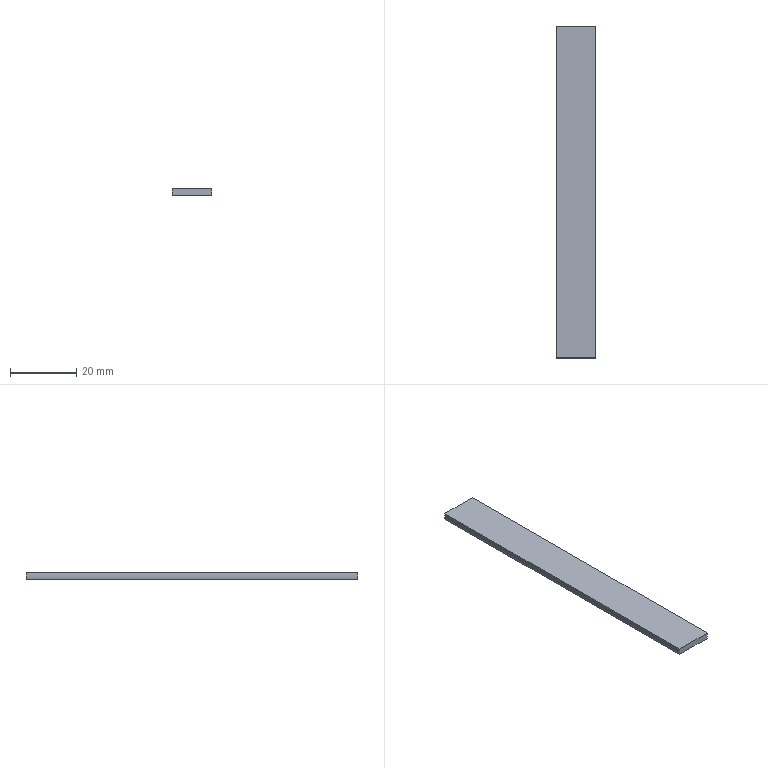Part | STEP file | Cooling fin - upper - Tower - 1 cav | 1 solid | 6 faces | box 12 x 100 x 2 mm | volume 2389 mm3 | plane 4 | cylinder 2 | commonest cylinder face diameters 12 x2
STEP:
#1=CARTESIAN_POINT('',(0.,0.,0.));
#2=DIRECTION('',(0.,0.,1.));
#3=DIRECTION('',(1.,0.,0.));
#4=AXIS2_PLACEMENT_3D('',#1,#2,#3);
#5=CARTESIAN_POINT('',(5.916,0.,-1.));
#6=VERTEX_POINT('',#5);
#7=CARTESIAN_POINT('',(5.916,100.,-1.));
#8=VERTEX_POINT('',#7);
#9=CARTESIAN_POINT('',(5.916,0.,-1.));
#10=DIRECTION('',(0.,1.,0.));
#11=VECTOR('',#10,1.);
#12=LINE('',#9,#11);
#13=CARTESIAN_POINT('',(-10.,100.,-1.));
#14=DIRECTION('',(0.,0.,1.));
#15=DIRECTION('',(1.,0.,0.));
#16=AXIS2_PLACEMENT_3D('',#13,#14,#15);
#17=PLANE('',#16);
#18=CARTESIAN_POINT('',(15.916,-100.));
#19=DIRECTION('',(0.,1.));
#20=VECTOR('',#19,1.);
#21=LINE('',#18,#20);
#22=(GEOMETRIC_REPRESENTATION_CONTEXT(2)PARAMETRIC_REPRESENTATION_CONTEXT()REPRESENTATION_CONTEXT('',''));
#23=DEFINITIONAL_REPRESENTATION('',(#21),#22);
#24=PCURVE('',#17,#23);
#25=CARTESIAN_POINT('',(0.,0.,0.));
#26=DIRECTION('',(0.,1.,0.));
#27=DIRECTION('',(0.,0.,1.));
#28=AXIS2_PLACEMENT_3D('',#25,#26,#27);
#29=CYLINDRICAL_SURFACE('',#28,6.);
#30=CARTESIAN_POINT('',(1.738,0.));
#31=DIRECTION('',(0.,1.));
#32=VECTOR('',#31,1.);
#33=LINE('',#30,#32);
#34=(GEOMETRIC_REPRESENTATION_CONTEXT(2)PARAMETRIC_REPRESENTATION_CONTEXT()REPRESENTATION_CONTEXT('',''));
#35=DEFINITIONAL_REPRESENTATION('',(#33),#34);
#36=PCURVE('',#29,#35);
#37=SURFACE_CURVE('',#12,(#24,#36),.PCURVE_S1.);
#38=EDGE_CURVE('',#6,#8,#37,.T.);
#39=ORIENTED_EDGE('',*,*,#38,.F.);
#40=CARTESIAN_POINT('',(-5.916,0.,-1.));
#41=VERTEX_POINT('',#40);
#42=CARTESIAN_POINT('',(-10.,0.,-1.));
#43=DIRECTION('',(-1.,0.,0.));
#44=VECTOR('',#43,1.);
#45=LINE('',#42,#44);
#46=CARTESIAN_POINT('',(0.,-100.));
#47=DIRECTION('',(-1.,0.));
#48=VECTOR('',#47,1.);
#49=LINE('',#46,#48);
#50=(GEOMETRIC_REPRESENTATION_CONTEXT(2)PARAMETRIC_REPRESENTATION_CONTEXT()REPRESENTATION_CONTEXT('',''));
#51=DEFINITIONAL_REPRESENTATION('',(#49),#50);
#52=PCURVE('',#17,#51);
#53=CARTESIAN_POINT('',(0.,0.,0.));
#54=DIRECTION('',(0.,-1.,0.));
#55=DIRECTION('',(0.,0.,-1.));
#56=AXIS2_PLACEMENT_3D('',#53,#54,#55);
#57=PLANE('',#56);
#58=CARTESIAN_POINT('',(1.,-10.));
#59=DIRECTION('',(0.,-1.));
#60=VECTOR('',#59,1.);
#61=LINE('',#58,#60);
#62=(GEOMETRIC_REPRESENTATION_CONTEXT(2)PARAMETRIC_REPRESENTATION_CONTEXT()REPRESENTATION_CONTEXT('',''));
#63=DEFINITIONAL_REPRESENTATION('',(#61),#62);
#64=PCURVE('',#57,#63);
#65=SURFACE_CURVE('',#45,(#52,#64),.PCURVE_S1.);
#66=EDGE_CURVE('',#6,#41,#65,.T.);
#67=ORIENTED_EDGE('',*,*,#66,.T.);
#68=CARTESIAN_POINT('',(-5.916,100.,-1.));
#69=VERTEX_POINT('',#68);
#70=CARTESIAN_POINT('',(-5.916,0.,-1.));
#71=DIRECTION('',(0.,-1.,0.));
#72=VECTOR('',#71,1.);
#73=LINE('',#70,#72);
#74=CARTESIAN_POINT('',(4.084,-100.));
#75=DIRECTION('',(0.,-1.));
#76=VECTOR('',#75,1.);
#77=LINE('',#74,#76);
#78=(GEOMETRIC_REPRESENTATION_CONTEXT(2)PARAMETRIC_REPRESENTATION_CONTEXT()REPRESENTATION_CONTEXT('',''));
#79=DEFINITIONAL_REPRESENTATION('',(#77),#78);
#80=PCURVE('',#17,#79);
#81=CARTESIAN_POINT('',(0.,0.,0.));
#82=DIRECTION('',(0.,1.,0.));
#83=DIRECTION('',(0.,0.,1.));
#84=AXIS2_PLACEMENT_3D('',#81,#82,#83);
#85=CYLINDRICAL_SURFACE('',#84,6.);
#86=CARTESIAN_POINT('',(4.545,0.));
#87=DIRECTION('',(0.,-1.));
#88=VECTOR('',#87,1.);
#89=LINE('',#86,#88);
#90=(GEOMETRIC_REPRESENTATION_CONTEXT(2)PARAMETRIC_REPRESENTATION_CONTEXT()REPRESENTATION_CONTEXT('',''));
#91=DEFINITIONAL_REPRESENTATION('',(#89),#90);
#92=PCURVE('',#85,#91);
#93=SURFACE_CURVE('',#73,(#80,#92),.PCURVE_S1.);
#94=EDGE_CURVE('',#69,#41,#93,.T.);
#95=ORIENTED_EDGE('',*,*,#94,.F.);
#96=CARTESIAN_POINT('',(-10.,100.,-1.));
#97=DIRECTION('',(-1.,0.,0.));
#98=VECTOR('',#97,1.);
#99=LINE('',#96,#98);
#100=CARTESIAN_POINT('',(0.,0.));
#101=DIRECTION('',(-1.,0.));
#102=VECTOR('',#101,1.);
#103=LINE('',#100,#102);
#104=(GEOMETRIC_REPRESENTATION_CONTEXT(2)PARAMETRIC_REPRESENTATION_CONTEXT()REPRESENTATION_CONTEXT('',''));
#105=DEFINITIONAL_REPRESENTATION('',(#103),#104);
#106=PCURVE('',#17,#105);
#107=CARTESIAN_POINT('',(0.,100.,0.));
#108=DIRECTION('',(0.,-1.,0.));
#109=DIRECTION('',(0.,0.,-1.));
#110=AXIS2_PLACEMENT_3D('',#107,#108,#109);
#111=PLANE('',#110);
#112=CARTESIAN_POINT('',(1.,-10.));
#113=DIRECTION('',(0.,-1.));
#114=VECTOR('',#113,1.);
#115=LINE('',#112,#114);
#116=(GEOMETRIC_REPRESENTATION_CONTEXT(2)PARAMETRIC_REPRESENTATION_CONTEXT()REPRESENTATION_CONTEXT('',''));
#117=DEFINITIONAL_REPRESENTATION('',(#115),#116);
#118=PCURVE('',#111,#117);
#119=SURFACE_CURVE('',#99,(#106,#118),.PCURVE_S1.);
#120=EDGE_CURVE('',#8,#69,#119,.T.);
#121=ORIENTED_EDGE('',*,*,#120,.F.);
#122=EDGE_LOOP('',(#39,#67,#95,#121));
#123=FACE_BOUND('',#122,.T.);
#124=ADVANCED_FACE('',(#123),#17,.F.);
#125=CARTESIAN_POINT('',(-5.916,0.,1.));
#126=VERTEX_POINT('',#125);
#127=CARTESIAN_POINT('',(-5.916,100.,1.));
#128=VERTEX_POINT('',#127);
#129=CARTESIAN_POINT('',(-5.916,0.,1.));
#130=DIRECTION('',(0.,1.,0.));
#131=VECTOR('',#130,1.);
#132=LINE('',#129,#131);
#133=CARTESIAN_POINT('',(-10.,100.,1.));
#134=DIRECTION('',(0.,0.,-1.));
#135=DIRECTION('',(-1.,0.,0.));
#136=AXIS2_PLACEMENT_3D('',#133,#134,#135);
#137=PLANE('',#136);
#138=CARTESIAN_POINT('',(-4.084,-100.));
#139=DIRECTION('',(0.,1.));
#140=VECTOR('',#139,1.);
#141=LINE('',#138,#140);
#142=(GEOMETRIC_REPRESENTATION_CONTEXT(2)PARAMETRIC_REPRESENTATION_CONTEXT()REPRESENTATION_CONTEXT('',''));
#143=DEFINITIONAL_REPRESENTATION('',(#141),#142);
#144=PCURVE('',#137,#143);
#145=CARTESIAN_POINT('',(4.88,0.));
#146=DIRECTION('',(0.,1.));
#147=VECTOR('',#146,1.);
#148=LINE('',#145,#147);
#149=(GEOMETRIC_REPRESENTATION_CONTEXT(2)PARAMETRIC_REPRESENTATION_CONTEXT()REPRESENTATION_CONTEXT('',''));
#150=DEFINITIONAL_REPRESENTATION('',(#148),#149);
#151=PCURVE('',#85,#150);
#152=SURFACE_CURVE('',#132,(#144,#151),.PCURVE_S1.);
#153=EDGE_CURVE('',#126,#128,#152,.T.);
#154=ORIENTED_EDGE('',*,*,#153,.F.);
#155=CARTESIAN_POINT('',(5.916,0.,1.));
#156=VERTEX_POINT('',#155);
#157=CARTESIAN_POINT('',(-10.,0.,1.));
#158=DIRECTION('',(1.,0.,0.));
#159=VECTOR('',#158,1.);
#160=LINE('',#157,#159);
#161=CARTESIAN_POINT('',(0.,-100.));
#162=DIRECTION('',(-1.,0.));
#163=VECTOR('',#162,1.);
#164=LINE('',#161,#163);
#165=(GEOMETRIC_REPRESENTATION_CONTEXT(2)PARAMETRIC_REPRESENTATION_CONTEXT()REPRESENTATION_CONTEXT('',''));
#166=DEFINITIONAL_REPRESENTATION('',(#164),#165);
#167=PCURVE('',#137,#166);
#168=CARTESIAN_POINT('',(-1.,-10.));
#169=DIRECTION('',(0.,1.));
#170=VECTOR('',#169,1.);
#171=LINE('',#168,#170);
#172=(GEOMETRIC_REPRESENTATION_CONTEXT(2)PARAMETRIC_REPRESENTATION_CONTEXT()REPRESENTATION_CONTEXT('',''));
#173=DEFINITIONAL_REPRESENTATION('',(#171),#172);
#174=PCURVE('',#57,#173);
#175=SURFACE_CURVE('',#160,(#167,#174),.PCURVE_S1.);
#176=EDGE_CURVE('',#126,#156,#175,.T.);
#177=ORIENTED_EDGE('',*,*,#176,.T.);
#178=CARTESIAN_POINT('',(5.916,100.,1.));
#179=VERTEX_POINT('',#178);
#180=CARTESIAN_POINT('',(5.916,0.,1.));
#181=DIRECTION('',(0.,-1.,0.));
#182=VECTOR('',#181,1.);
#183=LINE('',#180,#182);
#184=CARTESIAN_POINT('',(-15.916,-100.));
#185=DIRECTION('',(0.,-1.));
#186=VECTOR('',#185,1.);
#187=LINE('',#184,#186);
#188=(GEOMETRIC_REPRESENTATION_CONTEXT(2)PARAMETRIC_REPRESENTATION_CONTEXT()REPRESENTATION_CONTEXT('',''));
#189=DEFINITIONAL_REPRESENTATION('',(#187),#188);
#190=PCURVE('',#137,#189);
#191=CARTESIAN_POINT('',(1.403,0.));
#192=DIRECTION('',(0.,-1.));
#193=VECTOR('',#192,1.);
#194=LINE('',#191,#193);
#195=(GEOMETRIC_REPRESENTATION_CONTEXT(2)PARAMETRIC_REPRESENTATION_CONTEXT()REPRESENTATION_CONTEXT('',''));
#196=DEFINITIONAL_REPRESENTATION('',(#194),#195);
#197=PCURVE('',#29,#196);
#198=SURFACE_CURVE('',#183,(#190,#197),.PCURVE_S1.);
#199=EDGE_CURVE('',#179,#156,#198,.T.);
#200=ORIENTED_EDGE('',*,*,#199,.F.);
#201=CARTESIAN_POINT('',(-10.,100.,1.));
#202=DIRECTION('',(1.,0.,0.));
#203=VECTOR('',#202,1.);
#204=LINE('',#201,#203);
#205=CARTESIAN_POINT('',(0.,0.));
#206=DIRECTION('',(-1.,0.));
#207=VECTOR('',#206,1.);
#208=LINE('',#205,#207);
#209=(GEOMETRIC_REPRESENTATION_CONTEXT(2)PARAMETRIC_REPRESENTATION_CONTEXT()REPRESENTATION_CONTEXT('',''));
#210=DEFINITIONAL_REPRESENTATION('',(#208),#209);
#211=PCURVE('',#137,#210);
#212=CARTESIAN_POINT('',(-1.,-10.));
#213=DIRECTION('',(0.,1.));
#214=VECTOR('',#213,1.);
#215=LINE('',#212,#214);
#216=(GEOMETRIC_REPRESENTATION_CONTEXT(2)PARAMETRIC_REPRESENTATION_CONTEXT()REPRESENTATION_CONTEXT('',''));
#217=DEFINITIONAL_REPRESENTATION('',(#215),#216);
#218=PCURVE('',#111,#217);
#219=SURFACE_CURVE('',#204,(#211,#218),.PCURVE_S1.);
#220=EDGE_CURVE('',#128,#179,#219,.T.);
#221=ORIENTED_EDGE('',*,*,#220,.F.);
#222=EDGE_LOOP('',(#154,#177,#200,#221));
#223=FACE_BOUND('',#222,.T.);
#224=ADVANCED_FACE('',(#223),#137,.F.);
#225=CARTESIAN_POINT('',(0.,100.,0.));
#226=DIRECTION('',(0.,1.,0.));
#227=DIRECTION('',(0.,0.,1.));
#228=AXIS2_PLACEMENT_3D('',#225,#226,#227);
#229=CIRCLE('',#228,6.);
#230=CARTESIAN_POINT('',(-6.,0.));
#231=CARTESIAN_POINT('',(-6.,10.392));
#232=CARTESIAN_POINT('',(3.,5.196));
#233=CARTESIAN_POINT('',(12.,0.));
#234=CARTESIAN_POINT('',(3.,-5.196));
#235=CARTESIAN_POINT('',(-6.,-10.392));
#236=CARTESIAN_POINT('',(-6.,0.));
#237=(BOUNDED_CURVE()B_SPLINE_CURVE(2,(#230,#231,#232,#233,#234,#235,#236),.UNSPECIFIED.,.T.,.F.)B_SPLINE_CURVE_WITH_KNOTS((1,2,2,2,2,1),(-2.094,0.,2.094,4.189,6.283,8.378),.UNSPECIFIED.)CURVE()GEOMETRIC_REPRESENTATION_ITEM()RATIONAL_B_SPLINE_CURVE((1.,0.5,1.,0.5,1.,0.5,1.))REPRESENTATION_ITEM(''));
#238=(GEOMETRIC_REPRESENTATION_CONTEXT(2)PARAMETRIC_REPRESENTATION_CONTEXT()REPRESENTATION_CONTEXT('',''));
#239=DEFINITIONAL_REPRESENTATION('',(#237),#238);
#240=PCURVE('',#111,#239);
#241=CARTESIAN_POINT('',(0.,100.));
#242=DIRECTION('',(1.,0.));
#243=VECTOR('',#242,1.);
#244=LINE('',#241,#243);
#245=(GEOMETRIC_REPRESENTATION_CONTEXT(2)PARAMETRIC_REPRESENTATION_CONTEXT()REPRESENTATION_CONTEXT('',''));
#246=DEFINITIONAL_REPRESENTATION('',(#244),#245);
#247=PCURVE('',#29,#246);
#248=SURFACE_CURVE('',#229,(#240,#247),.PCURVE_S1.);
#249=EDGE_CURVE('',#179,#8,#248,.T.);
#250=ORIENTED_EDGE('',*,*,#249,.T.);
#251=ORIENTED_EDGE('',*,*,#120,.T.);
#252=CARTESIAN_POINT('',(0.,100.,0.));
#253=DIRECTION('',(0.,1.,0.));
#254=DIRECTION('',(0.,0.,1.));
#255=AXIS2_PLACEMENT_3D('',#252,#253,#254);
#256=CIRCLE('',#255,6.);
#257=CARTESIAN_POINT('',(-6.,0.));
#258=CARTESIAN_POINT('',(-6.,10.392));
#259=CARTESIAN_POINT('',(3.,5.196));
#260=CARTESIAN_POINT('',(12.,0.));
#261=CARTESIAN_POINT('',(3.,-5.196));
#262=CARTESIAN_POINT('',(-6.,-10.392));
#263=CARTESIAN_POINT('',(-6.,0.));
#264=(BOUNDED_CURVE()B_SPLINE_CURVE(2,(#257,#258,#259,#260,#261,#262,#263),.UNSPECIFIED.,.T.,.F.)B_SPLINE_CURVE_WITH_KNOTS((1,2,2,2,2,1),(-2.094,0.,2.094,4.189,6.283,8.378),.UNSPECIFIED.)CURVE()GEOMETRIC_REPRESENTATION_ITEM()RATIONAL_B_SPLINE_CURVE((1.,0.5,1.,0.5,1.,0.5,1.))REPRESENTATION_ITEM(''));
#265=(GEOMETRIC_REPRESENTATION_CONTEXT(2)PARAMETRIC_REPRESENTATION_CONTEXT()REPRESENTATION_CONTEXT('',''));
#266=DEFINITIONAL_REPRESENTATION('',(#264),#265);
#267=PCURVE('',#111,#266);
#268=CARTESIAN_POINT('',(0.,100.));
#269=DIRECTION('',(1.,0.));
#270=VECTOR('',#269,1.);
#271=LINE('',#268,#270);
#272=(GEOMETRIC_REPRESENTATION_CONTEXT(2)PARAMETRIC_REPRESENTATION_CONTEXT()REPRESENTATION_CONTEXT('',''));
#273=DEFINITIONAL_REPRESENTATION('',(#271),#272);
#274=PCURVE('',#85,#273);
#275=SURFACE_CURVE('',#256,(#267,#274),.PCURVE_S1.);
#276=EDGE_CURVE('',#69,#128,#275,.T.);
#277=ORIENTED_EDGE('',*,*,#276,.T.);
#278=ORIENTED_EDGE('',*,*,#220,.T.);
#279=EDGE_LOOP('',(#250,#251,#277,#278));
#280=FACE_BOUND('',#279,.T.);
#281=ADVANCED_FACE('',(#280),#111,.F.);
#282=ORIENTED_EDGE('',*,*,#66,.F.);
#283=CARTESIAN_POINT('',(0.,0.,0.));
#284=DIRECTION('',(0.,1.,0.));
#285=DIRECTION('',(0.,0.,1.));
#286=AXIS2_PLACEMENT_3D('',#283,#284,#285);
#287=CIRCLE('',#286,6.);
#288=CARTESIAN_POINT('',(-6.,0.));
#289=CARTESIAN_POINT('',(-6.,10.392));
#290=CARTESIAN_POINT('',(3.,5.196));
#291=CARTESIAN_POINT('',(12.,0.));
#292=CARTESIAN_POINT('',(3.,-5.196));
#293=CARTESIAN_POINT('',(-6.,-10.392));
#294=CARTESIAN_POINT('',(-6.,0.));
#295=(BOUNDED_CURVE()B_SPLINE_CURVE(2,(#288,#289,#290,#291,#292,#293,#294),.UNSPECIFIED.,.T.,.F.)B_SPLINE_CURVE_WITH_KNOTS((1,2,2,2,2,1),(-2.094,0.,2.094,4.189,6.283,8.378),.UNSPECIFIED.)CURVE()GEOMETRIC_REPRESENTATION_ITEM()RATIONAL_B_SPLINE_CURVE((1.,0.5,1.,0.5,1.,0.5,1.))REPRESENTATION_ITEM(''));
#296=(GEOMETRIC_REPRESENTATION_CONTEXT(2)PARAMETRIC_REPRESENTATION_CONTEXT()REPRESENTATION_CONTEXT('',''));
#297=DEFINITIONAL_REPRESENTATION('',(#295),#296);
#298=PCURVE('',#57,#297);
#299=CARTESIAN_POINT('',(0.,0.));
#300=DIRECTION('',(1.,0.));
#301=VECTOR('',#300,1.);
#302=LINE('',#299,#301);
#303=(GEOMETRIC_REPRESENTATION_CONTEXT(2)PARAMETRIC_REPRESENTATION_CONTEXT()REPRESENTATION_CONTEXT('',''));
#304=DEFINITIONAL_REPRESENTATION('',(#302),#303);
#305=PCURVE('',#29,#304);
#306=SURFACE_CURVE('',#287,(#298,#305),.PCURVE_S1.);
#307=EDGE_CURVE('',#156,#6,#306,.T.);
#308=ORIENTED_EDGE('',*,*,#307,.F.);
#309=ORIENTED_EDGE('',*,*,#176,.F.);
#310=CARTESIAN_POINT('',(0.,0.,0.));
#311=DIRECTION('',(0.,-1.,0.));
#312=DIRECTION('',(0.,0.,-1.));
#313=AXIS2_PLACEMENT_3D('',#310,#311,#312);
#314=CIRCLE('',#313,6.);
#315=CARTESIAN_POINT('',(0.,0.));
#316=DIRECTION('',(1.,0.));
#317=AXIS2_PLACEMENT_2D('',#315,#316);
#318=CIRCLE('',#317,6.);
#319=(GEOMETRIC_REPRESENTATION_CONTEXT(2)PARAMETRIC_REPRESENTATION_CONTEXT()REPRESENTATION_CONTEXT('',''));
#320=DEFINITIONAL_REPRESENTATION('',(#318),#319);
#321=PCURVE('',#57,#320);
#322=CARTESIAN_POINT('',(9.425,0.));
#323=DIRECTION('',(-1.,0.));
#324=VECTOR('',#323,1.);
#325=LINE('',#322,#324);
#326=(GEOMETRIC_REPRESENTATION_CONTEXT(2)PARAMETRIC_REPRESENTATION_CONTEXT()REPRESENTATION_CONTEXT('',''));
#327=DEFINITIONAL_REPRESENTATION('',(#325),#326);
#328=PCURVE('',#85,#327);
#329=SURFACE_CURVE('',#314,(#321,#328),.PCURVE_S1.);
#330=EDGE_CURVE('',#126,#41,#329,.T.);
#331=ORIENTED_EDGE('',*,*,#330,.T.);
#332=EDGE_LOOP('',(#282,#308,#309,#331));
#333=FACE_BOUND('',#332,.T.);
#334=ADVANCED_FACE('',(#333),#57,.T.);
#335=ORIENTED_EDGE('',*,*,#94,.T.);
#336=ORIENTED_EDGE('',*,*,#330,.F.);
#337=ORIENTED_EDGE('',*,*,#153,.T.);
#338=ORIENTED_EDGE('',*,*,#276,.F.);
#339=EDGE_LOOP('',(#335,#336,#337,#338));
#340=FACE_BOUND('',#339,.T.);
#341=ADVANCED_FACE('',(#340),#85,.T.);
#342=ORIENTED_EDGE('',*,*,#38,.T.);
#343=ORIENTED_EDGE('',*,*,#249,.F.);
#344=ORIENTED_EDGE('',*,*,#199,.T.);
#345=ORIENTED_EDGE('',*,*,#307,.T.);
#346=EDGE_LOOP('',(#342,#343,#344,#345));
#347=FACE_BOUND('',#346,.T.);
#348=ADVANCED_FACE('',(#347),#29,.T.);
#349=CLOSED_SHELL('',(#124,#224,#281,#334,#341,#348));
#350=MANIFOLD_SOLID_BREP('',#349);
#351=(LENGTH_UNIT()NAMED_UNIT(*)SI_UNIT(.MILLI.,.METRE.));
#352=UNCERTAINTY_MEASURE_WITH_UNIT(LENGTH_MEASURE(0.0000001),#351,'','');
#353=(NAMED_UNIT(*)PLANE_ANGLE_UNIT()SI_UNIT($,.RADIAN.));
#354=(NAMED_UNIT(*)SI_UNIT($,.STERADIAN.)SOLID_ANGLE_UNIT());
#355=(GEOMETRIC_REPRESENTATION_CONTEXT(3)GLOBAL_UNCERTAINTY_ASSIGNED_CONTEXT((#352))GLOBAL_UNIT_ASSIGNED_CONTEXT((#351,#353,#354))REPRESENTATION_CONTEXT('',''));
#356=ADVANCED_BREP_SHAPE_REPRESENTATION('',(#4,#350),#355);